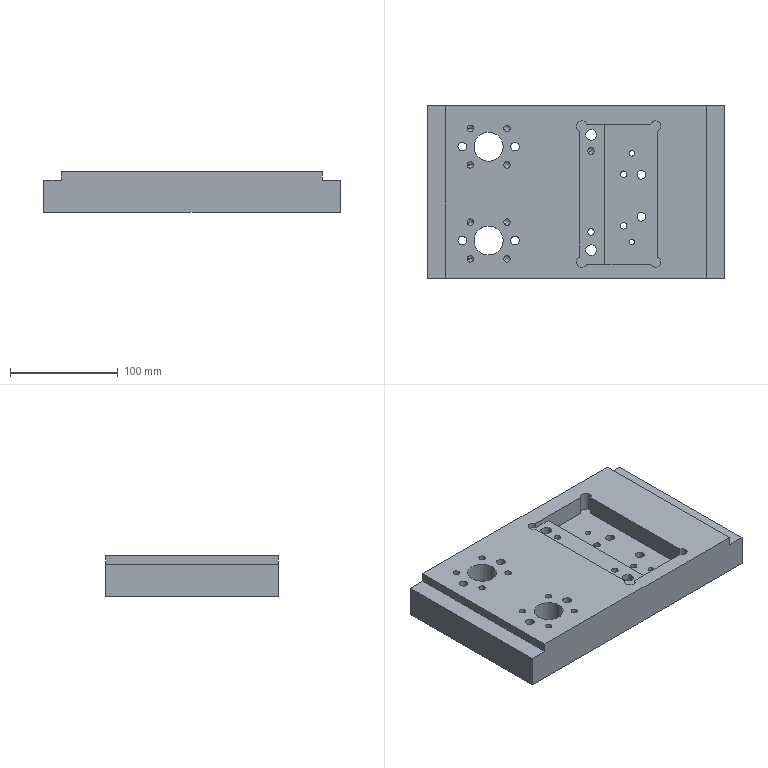Part | 1 solid | 87 faces | box 275.4 x 160 x 38 mm | volume 1435532 mm3 | cylinder 52 | cone 18 | plane 17 | commonest cylinder face diameters 6 x24 8 x12 5 x4 10 x4 10.02 x4 27 x4